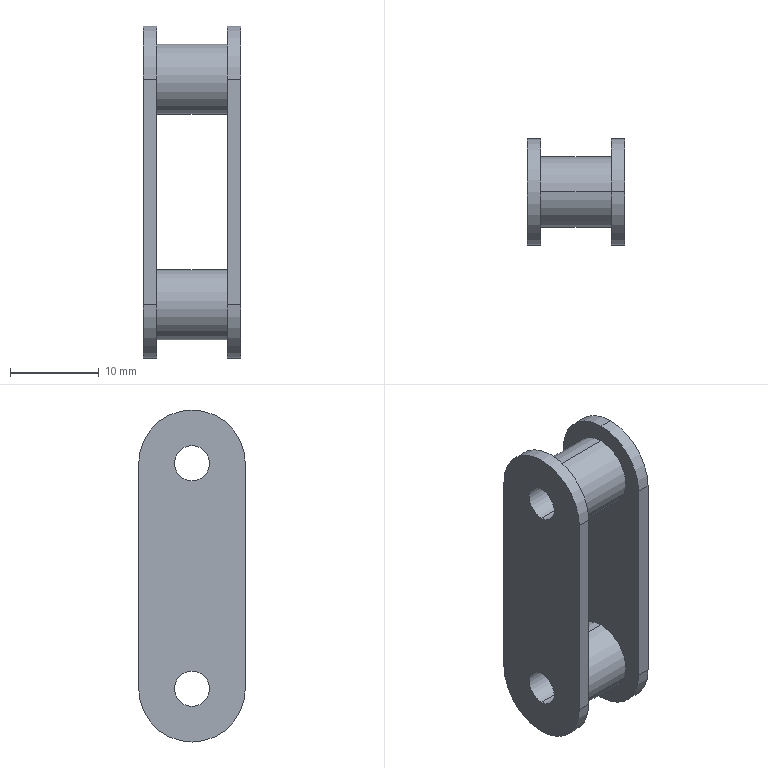Part | STEP file | 0228_Z_Chain_RF2040SSS-442 | 1 solid | 22 faces | box 10.95 x 12 x 37.4 mm | volume 1766 mm3 | cylinder 14 | plane 8 | commonest cylinder face diameters 12 x6 3.97 x4 7.92 x4